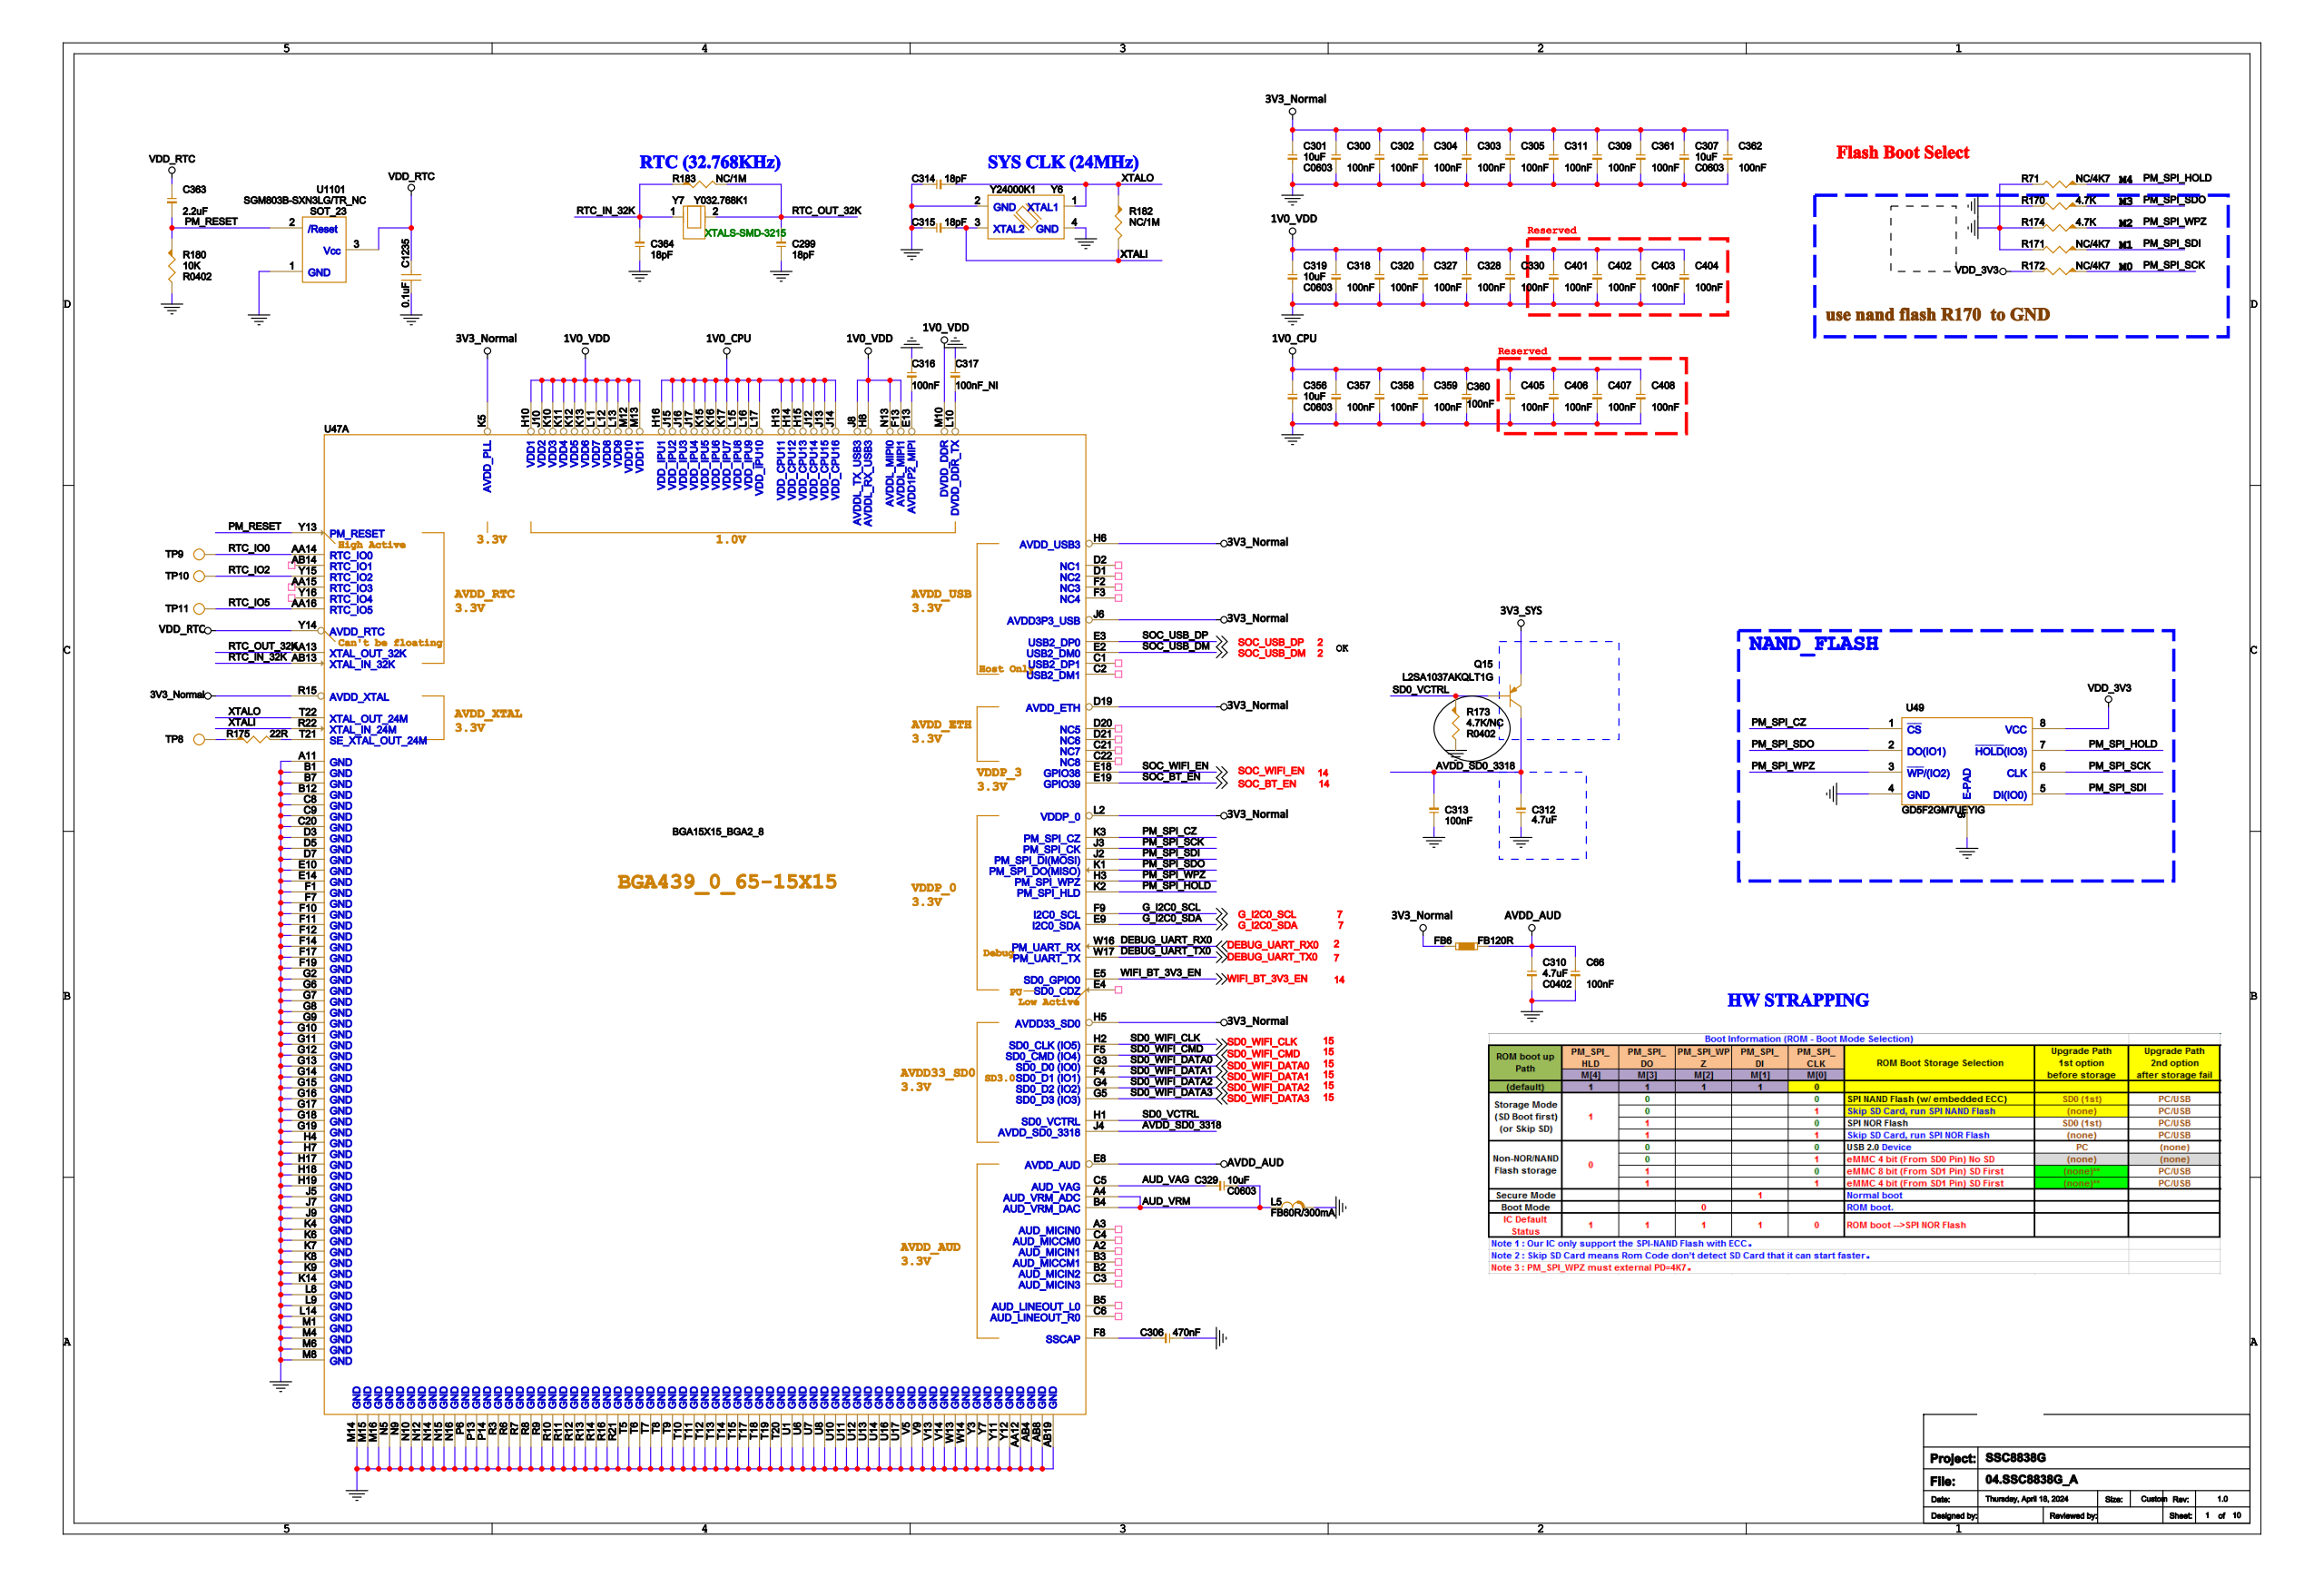Circuit board | Cadence Allegro | 958 parts | 601 nets | one sheet of the schematic
Parts on this sheet (reference | value | footprint):
C66 | 100nF | C0402
C299 | 18pF | C0402
C300 | 100nF | C0402
C301 | 10uF | C0603
C302 | 100nF | C0402
C303 | 100nF | C0402
C304 | 100nF | C0402
C305 | 100nF | C0402
C306 | 470nF | C0402
C307 | 10uF | C0603
C309 | 100nF | C0402
C310 | 4.7uF | C0402
C311 | 100nF | C0402
C312 | 4.7uF | C0402
C313 | 100nF | C0402
C314 | 18pF | C0402
C315 | 18pF | C0402
C316 | 100nF | C0402
C317 | 100nF_NI | C0402
C318 | 100nF | C0402
C319 | 10uF | C0603
C320 | 100nF | C0402
C327 | 100nF | C0402
C328 | 100nF | C0402
C329 | 10uF | C0603
C330 | 100nF | C0402
C356 | 10uF | C0603
C357 | 100nF | C0402
C358 | 100nF | C0402
C359 | 100nF | C0402
C360 | 100nF | C0402
C361 | 100nF | C0402
C362 | 100nF | C0402
C363 | 2.2uF | C0402
C364 | 18pF | C0402
C401 | 100nF | C0402
C402 | 100nF | C0402
C403 | 100nF | C0402
C404 | 100nF | C0402
C405 | 100nF | C0402
C406 | 100nF | C0402
C407 | 100nF | C0402
C408 | 100nF | C0402
C1235 | 0.1uF | C0402
FB6 | FB120R | L0402
L5 | FB60R/300mA | L0402
Q15 | L2SA1037AKQLT1G | SOT-23
R71 | NC/4K7 | R0402
R170 | 4.7K | R0402
R171 | NC/4K7 | R0402
R172 | NC/4K7 | R0402
R173 | 4.7K/NC | R0402
R174 | 4.7K | R0402
R175 | 22R | R0402
R180 | 10K | R0402
R182 | NC/1M | R0402
R183 | NC/1M | R0402
TP8 | Test_Point | TP_0R50
TP9 | Test_Point | TP_0R50
TP10 | Test_Point | TP_0R50
TP11 | Test_Point | TP_0R50
U47 | BGA15X15_BGA2_8 | 8838G
U49 | GD5F2GM7UEYIG | GD25-SOP8-WSON8
U1101 | SGM803B-SXN3LG/TR_NC | SOT_23
Y6 | Y24000K1 | TCXO-3225
Y7 | Y032.768K1 | XTALS-SMD-3215
Nets of these parts (net: part-pin ...):
GND: C66-2 C299-1 C300-2 C301-1 C302-2 C303-2 C304-2 C305-2 C306-1 C307-1 C309-2 C310-1 C311-2 C312-2 C313-1 C314-1 C315-1 C316-1 C317-1 C318-2 C319-1 C320-2 C327-2 C328-2 C330-2 C356-1 C357-2 C358-2 C359-2 C360-2 C361-2 C362-2 C364-1 C401-2 C402-2 C403-2 C404-2 C405-2 C406-2 C407-2 C408-2 C1235-1 L5-1 R71-2 R170-2 R171-2 R173-2 R174-2 R180-2 U49-4 U49-9 U1101-1 Y6-2 Y6-4 U47-A11 U47-AA12 U47-AB4 U47-AB8 U47-AB19 U47-B1 U47-B7 U47-B12 U47-C8 U47-C9 U47-C20 U47-D3 U47-D5 U47-D7 U47-E10 U47-E14 U47-F1 U47-F7 U47-F10 U47-F11 U47-F12 U47-F14 U47-F17 U47-F19 U47-G2 U47-G6 U47-G7 U47-G8 U47-G9 U47-G10 U47-G11 U47-G12 U47-G13 U47-G14 U47-G15 U47-G16 U47-G17 U47-G18 U47-G19 U47-H4 U47-H7 U47-H17 U47-H18 U47-H19 U47-J5 U47-J7 U47-J9 U47-K4 U47-K6 U47-K7 U47-K8 U47-K9 U47-K14 U47-L8 U47-L9 U47-L14 U47-M1 U47-M4 U47-M6 U47-M8 U47-M14 U47-M15 U47-M16 U47-N5 U47-N9 U47-N10 U47-N12 U47-N14 U47-N15 U47-N16 U47-P6 U47-P13 U47-P14 U47-R3 U47-R6 U47-R7 U47-R8 U47-R9 U47-R10 U47-R11 U47-R12 U47-R13 U47-R14 U47-R16 U47-R21 U47-T5 U47-T6 U47-T7 U47-T8 U47-T9 U47-T10 U47-T11 U47-T12 U47-T13 U47-T14 U47-T15 U47-T17 U47-T18 U47-T19 U47-T20 U47-U1 U47-U6 U47-U7 U47-U8 U47-U10 U47-U11 U47-U12 U47-U13 U47-U14 U47-U16 U47-U17 U47-V5 U47-V9 U47-V13 U47-V14 U47-W13 U47-W14 U47-Y3 U47-Y7 U47-Y11 U47-Y12
3V3_NORMAL: C300-1 C301-2 C302-1 C303-1 C304-1 C305-1 C307-2 C309-1 C311-1 C361-1 C362-1 FB6-1 Q15-2 R172-2 U49-8 U47-D19 U47-H5 U47-H6 U47-J6 U47-K5 U47-L2 U47-R15
AVDD_SD0_3318: C312-1 C313-2 Q15-3 U47-J4
N20521025: C316-2 U47-E13
1V0_VDD: C318-1 C319-2 C320-1 C327-1 C328-1 C330-1 C401-1 C402-1 C403-1 C404-1 U47-F13 U47-H8 U47-H10 U47-J8 U47-J10 U47-K10 U47-K11 U47-K12 U47-K13 U47-L11 U47-L12 U47-L13 U47-M10 U47-M12 U47-M13 U47-N13
1V0_CPU: C356-2 C357-1 C358-1 C359-1 C360-1 C405-1 C406-1 C407-1 C408-1 U47-H13 U47-H14 U47-H15 U47-H16 U47-J12 U47-J13 U47-J14 U47-J15 U47-J16 U47-J17 U47-K15 U47-K16 U47-K17 U47-L15 U47-L16 U47-L17
AVDD_AUD: C66-1 C310-2 FB6-2 U47-E8
VDD_RTC: C363-1 C1235-2 U1101-3 U47-Y14
SD0_WIFI_CLK: U47-H2
RTC_OUT_32K: C299-2 R183-2 Y7-2 U47-AA13
XTALO: C314-2 R182-1 Y6-1 U47-T22
XTALI: C315-2 R182-2 Y6-3 U47-R22
RTC_IN_32K: C364-2 R183-1 Y7-1 U47-AB13
N20521414: C306-2 U47-F8
N20522459: C317-2 U47-L10
AUD_VAG: C329-1 U47-C5
AUD_VRM: C329-2 L5-2 U47-A4 U47-B4
PM_RESET: C363-2 R180-1 U1101-2 U47-Y13
SOC_USB_DM: U47-E2
SOC_USB_DP: U47-E3
SD0_VCTRL: Q15-1 R173-1 U47-H1
PM_SPI_SDO: R170-1 U49-2 U47-K1
PM_SPI_WPZ: R174-1 U49-3 U47-H3
PM_SPI_SDI: R171-1 U49-5 U47-J2
PM_SPI_SCK: R172-1 U49-6 U47-J3
PM_SPI_HOLD: R71-1 U49-7 U47-K2
N20521999: R175-1 TP8-1
N20522413: R175-2 U47-T21
G_I2C0_SCL: U47-F9
G_I2C0_SDA: U47-E9
SOC_BT_EN: U47-E19
SOC_WIFI_EN: U47-E18
SD0_WIFI_DATA0: U47-G3
SD0_WIFI_DATA1: U47-F4
SD0_WIFI_DATA2: U47-G4
SD0_WIFI_DATA3: U47-G5
SD0_WIFI_CMD: U47-F5
DEBUG_UART_TX0: U47-W17
DEBUG_UART_RX0: U47-W16
WIFI_BT_3V3_EN: U47-E5
RTC_IO2: TP10-1 U47-Y15
RTC_IO5: TP11-1 U47-AA16
RTC_IO0: TP9-1 U47-AA14
PM_SPI_CZ: U49-1 U47-K3